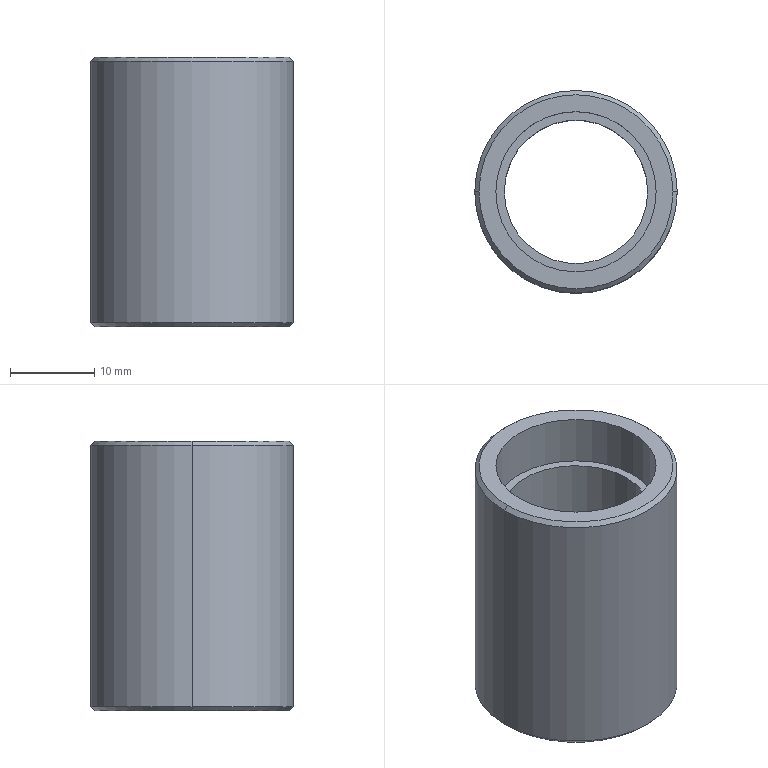Part | STEP file | QA-FC01 | 1 solid | 16 faces | box 24 x 24 x 32 mm | volume 6516 mm3 | cylinder 8 | cone 4 | plane 4 | commonest cylinder face diameters 19 x4 17 x2 24 x2
STEP:
#1=CARTESIAN_POINT('',(0.,0.,0.));
#2=DIRECTION('',(0.,0.,1.));
#3=DIRECTION('',(1.,0.,0.));
#4=AXIS2_PLACEMENT_3D('',#1,#2,#3);
#5=CARTESIAN_POINT('',(11.5,0.,32.));
#6=VERTEX_POINT('',#5);
#7=CARTESIAN_POINT('',(-11.5,0.,32.));
#8=VERTEX_POINT('',#7);
#9=CARTESIAN_POINT('',(0.,0.,32.));
#10=DIRECTION('',(0.,0.,1.));
#11=DIRECTION('',(1.,0.,0.));
#12=AXIS2_PLACEMENT_3D('',#9,#10,#11);
#13=CIRCLE('',#12,11.5);
#14=CARTESIAN_POINT('',(0.,0.,32.));
#15=DIRECTION('',(0.,0.,-1.));
#16=DIRECTION('',(-1.,0.,0.));
#17=AXIS2_PLACEMENT_3D('',#14,#15,#16);
#18=CONICAL_SURFACE('',#17,11.5,0.7854);
#19=CARTESIAN_POINT('',(3.142,0.));
#20=DIRECTION('',(-1.,0.));
#21=VECTOR('',#20,1.);
#22=LINE('',#19,#21);
#23=(GEOMETRIC_REPRESENTATION_CONTEXT(2)PARAMETRIC_REPRESENTATION_CONTEXT()REPRESENTATION_CONTEXT('',''));
#24=DEFINITIONAL_REPRESENTATION('',(#22),#23);
#25=PCURVE('',#18,#24);
#26=CARTESIAN_POINT('',(0.,0.,32.));
#27=DIRECTION('',(0.,0.,1.));
#28=DIRECTION('',(1.,0.,0.));
#29=AXIS2_PLACEMENT_3D('',#26,#27,#28);
#30=PLANE('',#29);
#31=CARTESIAN_POINT('',(0.,0.));
#32=DIRECTION('',(1.,0.));
#33=AXIS2_PLACEMENT_2D('',#31,#32);
#34=CIRCLE('',#33,11.5);
#35=(GEOMETRIC_REPRESENTATION_CONTEXT(2)PARAMETRIC_REPRESENTATION_CONTEXT()REPRESENTATION_CONTEXT('',''));
#36=DEFINITIONAL_REPRESENTATION('',(#34),#35);
#37=PCURVE('',#30,#36);
#38=SURFACE_CURVE('',#13,(#25,#37),.PCURVE_S1.);
#39=EDGE_CURVE('',#6,#8,#38,.T.);
#40=ORIENTED_EDGE('',*,*,#39,.F.);
#41=CARTESIAN_POINT('',(12.,0.,31.5));
#42=VERTEX_POINT('',#41);
#43=CARTESIAN_POINT('',(11.5,0.,32.));
#44=DIRECTION('',(0.7071,0.,-0.7071));
#45=VECTOR('',#44,1.);
#46=LINE('',#43,#45);
#47=CARTESIAN_POINT('',(3.142,0.));
#48=DIRECTION('',(0.,1.));
#49=VECTOR('',#48,1.);
#50=LINE('',#47,#49);
#51=(GEOMETRIC_REPRESENTATION_CONTEXT(2)PARAMETRIC_REPRESENTATION_CONTEXT()REPRESENTATION_CONTEXT('',''));
#52=DEFINITIONAL_REPRESENTATION('',(#50),#51);
#53=PCURVE('',#18,#52);
#54=CARTESIAN_POINT('',(0.,0.,32.));
#55=DIRECTION('',(0.,0.,-1.));
#56=DIRECTION('',(-1.,0.,0.));
#57=AXIS2_PLACEMENT_3D('',#54,#55,#56);
#58=CONICAL_SURFACE('',#57,11.5,0.7854);
#59=CARTESIAN_POINT('',(3.142,0.));
#60=DIRECTION('',(0.,1.));
#61=VECTOR('',#60,1.);
#62=LINE('',#59,#61);
#63=(GEOMETRIC_REPRESENTATION_CONTEXT(2)PARAMETRIC_REPRESENTATION_CONTEXT()REPRESENTATION_CONTEXT('',''));
#64=DEFINITIONAL_REPRESENTATION('',(#62),#63);
#65=PCURVE('',#58,#64);
#66=SURFACE_CURVE('',#46,(#53,#65),.PCURVE_S1.);
#67=EDGE_CURVE('',#6,#42,#66,.T.);
#68=ORIENTED_EDGE('',*,*,#67,.T.);
#69=CARTESIAN_POINT('',(-12.,0.,31.5));
#70=VERTEX_POINT('',#69);
#71=CARTESIAN_POINT('',(0.,0.,31.5));
#72=DIRECTION('',(0.,0.,-1.));
#73=DIRECTION('',(1.,0.,0.));
#74=AXIS2_PLACEMENT_3D('',#71,#72,#73);
#75=CIRCLE('',#74,12.);
#76=CARTESIAN_POINT('',(-3.142,0.5));
#77=DIRECTION('',(1.,0.));
#78=VECTOR('',#77,1.);
#79=LINE('',#76,#78);
#80=(GEOMETRIC_REPRESENTATION_CONTEXT(2)PARAMETRIC_REPRESENTATION_CONTEXT()REPRESENTATION_CONTEXT('',''));
#81=DEFINITIONAL_REPRESENTATION('',(#79),#80);
#82=PCURVE('',#18,#81);
#83=CARTESIAN_POINT('',(0.,0.,32.));
#84=DIRECTION('',(0.,0.,-1.));
#85=DIRECTION('',(-1.,0.,0.));
#86=AXIS2_PLACEMENT_3D('',#83,#84,#85);
#87=CYLINDRICAL_SURFACE('',#86,12.);
#88=CARTESIAN_POINT('',(-3.142,0.5));
#89=DIRECTION('',(1.,0.));
#90=VECTOR('',#89,1.);
#91=LINE('',#88,#90);
#92=(GEOMETRIC_REPRESENTATION_CONTEXT(2)PARAMETRIC_REPRESENTATION_CONTEXT()REPRESENTATION_CONTEXT('',''));
#93=DEFINITIONAL_REPRESENTATION('',(#91),#92);
#94=PCURVE('',#87,#93);
#95=SURFACE_CURVE('',#75,(#82,#94),.PCURVE_S1.);
#96=EDGE_CURVE('',#70,#42,#95,.T.);
#97=ORIENTED_EDGE('',*,*,#96,.F.);
#98=CARTESIAN_POINT('',(-11.5,0.,32.));
#99=DIRECTION('',(-0.7071,0.,-0.7071));
#100=VECTOR('',#99,1.);
#101=LINE('',#98,#100);
#102=CARTESIAN_POINT('',(0.,0.));
#103=DIRECTION('',(0.,1.));
#104=VECTOR('',#103,1.);
#105=LINE('',#102,#104);
#106=(GEOMETRIC_REPRESENTATION_CONTEXT(2)PARAMETRIC_REPRESENTATION_CONTEXT()REPRESENTATION_CONTEXT('',''));
#107=DEFINITIONAL_REPRESENTATION('',(#105),#106);
#108=PCURVE('',#18,#107);
#109=CARTESIAN_POINT('',(6.283,0.));
#110=DIRECTION('',(0.,1.));
#111=VECTOR('',#110,1.);
#112=LINE('',#109,#111);
#113=(GEOMETRIC_REPRESENTATION_CONTEXT(2)PARAMETRIC_REPRESENTATION_CONTEXT()REPRESENTATION_CONTEXT('',''));
#114=DEFINITIONAL_REPRESENTATION('',(#112),#113);
#115=PCURVE('',#58,#114);
#116=SURFACE_CURVE('',#101,(#108,#115),.PCURVE_S1.);
#117=EDGE_CURVE('',#8,#70,#116,.T.);
#118=ORIENTED_EDGE('',*,*,#117,.F.);
#119=EDGE_LOOP('',(#40,#68,#97,#118));
#120=FACE_BOUND('',#119,.T.);
#121=ADVANCED_FACE('',(#120),#18,.T.);
#122=CARTESIAN_POINT('',(-11.5,0.,0.));
#123=VERTEX_POINT('',#122);
#124=CARTESIAN_POINT('',(11.5,0.,0.));
#125=VERTEX_POINT('',#124);
#126=CARTESIAN_POINT('',(0.,0.,0.));
#127=DIRECTION('',(0.,0.,-1.));
#128=DIRECTION('',(1.,0.,0.));
#129=AXIS2_PLACEMENT_3D('',#126,#127,#128);
#130=CIRCLE('',#129,11.5);
#131=CARTESIAN_POINT('',(0.,0.,0.5));
#132=DIRECTION('',(0.,0.,1.));
#133=DIRECTION('',(1.,0.,0.));
#134=AXIS2_PLACEMENT_3D('',#131,#132,#133);
#135=CONICAL_SURFACE('',#134,12.,0.7854);
#136=CARTESIAN_POINT('',(6.283,-0.5));
#137=DIRECTION('',(-1.,0.));
#138=VECTOR('',#137,1.);
#139=LINE('',#136,#138);
#140=(GEOMETRIC_REPRESENTATION_CONTEXT(2)PARAMETRIC_REPRESENTATION_CONTEXT()REPRESENTATION_CONTEXT('',''));
#141=DEFINITIONAL_REPRESENTATION('',(#139),#140);
#142=PCURVE('',#135,#141);
#143=CARTESIAN_POINT('',(0.,0.,0.));
#144=DIRECTION('',(0.,0.,1.));
#145=DIRECTION('',(1.,0.,0.));
#146=AXIS2_PLACEMENT_3D('',#143,#144,#145);
#147=PLANE('',#146);
#148=CARTESIAN_POINT('',(11.5,0.));
#149=CARTESIAN_POINT('',(11.5,-19.919));
#150=CARTESIAN_POINT('',(-5.75,-9.959));
#151=CARTESIAN_POINT('',(-23.,0.));
#152=CARTESIAN_POINT('',(-5.75,9.959));
#153=CARTESIAN_POINT('',(11.5,19.919));
#154=CARTESIAN_POINT('',(11.5,0.));
#155=(BOUNDED_CURVE()B_SPLINE_CURVE(2,(#148,#149,#150,#151,#152,#153,#154),.UNSPECIFIED.,.T.,.F.)B_SPLINE_CURVE_WITH_KNOTS((1,2,2,2,2,1),(-2.094,0.,2.094,4.189,6.283,8.378),.UNSPECIFIED.)CURVE()GEOMETRIC_REPRESENTATION_ITEM()RATIONAL_B_SPLINE_CURVE((1.,0.5,1.,0.5,1.,0.5,1.))REPRESENTATION_ITEM(''));
#156=(GEOMETRIC_REPRESENTATION_CONTEXT(2)PARAMETRIC_REPRESENTATION_CONTEXT()REPRESENTATION_CONTEXT('',''));
#157=DEFINITIONAL_REPRESENTATION('',(#155),#156);
#158=PCURVE('',#147,#157);
#159=SURFACE_CURVE('',#130,(#142,#158),.PCURVE_S1.);
#160=EDGE_CURVE('',#123,#125,#159,.T.);
#161=ORIENTED_EDGE('',*,*,#160,.F.);
#162=CARTESIAN_POINT('',(-12.,0.,0.5));
#163=VERTEX_POINT('',#162);
#164=CARTESIAN_POINT('',(-12.,0.,0.5));
#165=DIRECTION('',(-0.7071,0.,0.7071));
#166=VECTOR('',#165,1.);
#167=LINE('',#164,#166);
#168=CARTESIAN_POINT('',(3.142,0.));
#169=DIRECTION('',(0.,1.));
#170=VECTOR('',#169,1.);
#171=LINE('',#168,#170);
#172=(GEOMETRIC_REPRESENTATION_CONTEXT(2)PARAMETRIC_REPRESENTATION_CONTEXT()REPRESENTATION_CONTEXT('',''));
#173=DEFINITIONAL_REPRESENTATION('',(#171),#172);
#174=PCURVE('',#135,#173);
#175=CARTESIAN_POINT('',(0.,0.,0.5));
#176=DIRECTION('',(0.,0.,1.));
#177=DIRECTION('',(1.,0.,0.));
#178=AXIS2_PLACEMENT_3D('',#175,#176,#177);
#179=CONICAL_SURFACE('',#178,12.,0.7854);
#180=CARTESIAN_POINT('',(3.142,0.));
#181=DIRECTION('',(0.,1.));
#182=VECTOR('',#181,1.);
#183=LINE('',#180,#182);
#184=(GEOMETRIC_REPRESENTATION_CONTEXT(2)PARAMETRIC_REPRESENTATION_CONTEXT()REPRESENTATION_CONTEXT('',''));
#185=DEFINITIONAL_REPRESENTATION('',(#183),#184);
#186=PCURVE('',#179,#185);
#187=SURFACE_CURVE('',#167,(#174,#186),.PCURVE_S1.);
#188=EDGE_CURVE('',#123,#163,#187,.T.);
#189=ORIENTED_EDGE('',*,*,#188,.T.);
#190=CARTESIAN_POINT('',(12.,0.,0.5));
#191=VERTEX_POINT('',#190);
#192=CARTESIAN_POINT('',(0.,0.,0.5));
#193=DIRECTION('',(0.,0.,1.));
#194=DIRECTION('',(1.,0.,0.));
#195=AXIS2_PLACEMENT_3D('',#192,#193,#194);
#196=CIRCLE('',#195,12.);
#197=CARTESIAN_POINT('',(0.,0.));
#198=DIRECTION('',(1.,0.));
#199=VECTOR('',#198,1.);
#200=LINE('',#197,#199);
#201=(GEOMETRIC_REPRESENTATION_CONTEXT(2)PARAMETRIC_REPRESENTATION_CONTEXT()REPRESENTATION_CONTEXT('',''));
#202=DEFINITIONAL_REPRESENTATION('',(#200),#201);
#203=PCURVE('',#135,#202);
#204=CARTESIAN_POINT('',(3.142,31.5));
#205=DIRECTION('',(-1.,0.));
#206=VECTOR('',#205,1.);
#207=LINE('',#204,#206);
#208=(GEOMETRIC_REPRESENTATION_CONTEXT(2)PARAMETRIC_REPRESENTATION_CONTEXT()REPRESENTATION_CONTEXT('',''));
#209=DEFINITIONAL_REPRESENTATION('',(#207),#208);
#210=PCURVE('',#87,#209);
#211=SURFACE_CURVE('',#196,(#203,#210),.PCURVE_S1.);
#212=EDGE_CURVE('',#191,#163,#211,.T.);
#213=ORIENTED_EDGE('',*,*,#212,.F.);
#214=CARTESIAN_POINT('',(12.,0.,0.5));
#215=DIRECTION('',(0.7071,0.,0.7071));
#216=VECTOR('',#215,1.);
#217=LINE('',#214,#216);
#218=CARTESIAN_POINT('',(0.,0.));
#219=DIRECTION('',(0.,1.));
#220=VECTOR('',#219,1.);
#221=LINE('',#218,#220);
#222=(GEOMETRIC_REPRESENTATION_CONTEXT(2)PARAMETRIC_REPRESENTATION_CONTEXT()REPRESENTATION_CONTEXT('',''));
#223=DEFINITIONAL_REPRESENTATION('',(#221),#222);
#224=PCURVE('',#135,#223);
#225=CARTESIAN_POINT('',(6.283,0.));
#226=DIRECTION('',(0.,1.));
#227=VECTOR('',#226,1.);
#228=LINE('',#225,#227);
#229=(GEOMETRIC_REPRESENTATION_CONTEXT(2)PARAMETRIC_REPRESENTATION_CONTEXT()REPRESENTATION_CONTEXT('',''));
#230=DEFINITIONAL_REPRESENTATION('',(#228),#229);
#231=PCURVE('',#179,#230);
#232=SURFACE_CURVE('',#217,(#224,#231),.PCURVE_S1.);
#233=EDGE_CURVE('',#125,#191,#232,.T.);
#234=ORIENTED_EDGE('',*,*,#233,.F.);
#235=EDGE_LOOP('',(#161,#189,#213,#234));
#236=FACE_BOUND('',#235,.T.);
#237=ADVANCED_FACE('',(#236),#135,.T.);
#238=CARTESIAN_POINT('',(-9.5,0.,6.));
#239=VERTEX_POINT('',#238);
#240=CARTESIAN_POINT('',(-9.5,0.,0.));
#241=VERTEX_POINT('',#240);
#242=CARTESIAN_POINT('',(-9.5,0.,6.));
#243=DIRECTION('',(0.,0.,-1.));
#244=VECTOR('',#243,1.);
#245=LINE('',#242,#244);
#246=CARTESIAN_POINT('',(0.,0.,6.));
#247=DIRECTION('',(0.,0.,-1.));
#248=DIRECTION('',(-1.,0.,0.));
#249=AXIS2_PLACEMENT_3D('',#246,#247,#248);
#250=CYLINDRICAL_SURFACE('',#249,9.5);
#251=CARTESIAN_POINT('',(6.283,0.));
#252=DIRECTION('',(0.,1.));
#253=VECTOR('',#252,1.);
#254=LINE('',#251,#253);
#255=(GEOMETRIC_REPRESENTATION_CONTEXT(2)PARAMETRIC_REPRESENTATION_CONTEXT()REPRESENTATION_CONTEXT('',''));
#256=DEFINITIONAL_REPRESENTATION('',(#254),#255);
#257=PCURVE('',#250,#256);
#258=CARTESIAN_POINT('',(0.,0.,6.));
#259=DIRECTION('',(0.,0.,-1.));
#260=DIRECTION('',(-1.,0.,0.));
#261=AXIS2_PLACEMENT_3D('',#258,#259,#260);
#262=CYLINDRICAL_SURFACE('',#261,9.5);
#263=CARTESIAN_POINT('',(0.,0.));
#264=DIRECTION('',(0.,1.));
#265=VECTOR('',#264,1.);
#266=LINE('',#263,#265);
#267=(GEOMETRIC_REPRESENTATION_CONTEXT(2)PARAMETRIC_REPRESENTATION_CONTEXT()REPRESENTATION_CONTEXT('',''));
#268=DEFINITIONAL_REPRESENTATION('',(#266),#267);
#269=PCURVE('',#262,#268);
#270=SURFACE_CURVE('',#245,(#257,#269),.PCURVE_S1.);
#271=EDGE_CURVE('',#239,#241,#270,.T.);
#272=ORIENTED_EDGE('',*,*,#271,.T.);
#273=CARTESIAN_POINT('',(9.5,0.,0.));
#274=VERTEX_POINT('',#273);
#275=CARTESIAN_POINT('',(0.,0.,0.));
#276=DIRECTION('',(0.,0.,-1.));
#277=DIRECTION('',(-1.,0.,0.));
#278=AXIS2_PLACEMENT_3D('',#275,#276,#277);
#279=CIRCLE('',#278,9.5);
#280=CARTESIAN_POINT('',(0.,6.));
#281=DIRECTION('',(1.,0.));
#282=VECTOR('',#281,1.);
#283=LINE('',#280,#282);
#284=(GEOMETRIC_REPRESENTATION_CONTEXT(2)PARAMETRIC_REPRESENTATION_CONTEXT()REPRESENTATION_CONTEXT('',''));
#285=DEFINITIONAL_REPRESENTATION('',(#283),#284);
#286=PCURVE('',#250,#285);
#287=CARTESIAN_POINT('',(-9.5,0.));
#288=CARTESIAN_POINT('',(-9.5,16.454));
#289=CARTESIAN_POINT('',(4.75,8.227));
#290=CARTESIAN_POINT('',(19.,0.));
#291=CARTESIAN_POINT('',(4.75,-8.227));
#292=CARTESIAN_POINT('',(-9.5,-16.454));
#293=CARTESIAN_POINT('',(-9.5,0.));
#294=(BOUNDED_CURVE()B_SPLINE_CURVE(2,(#287,#288,#289,#290,#291,#292,#293),.UNSPECIFIED.,.T.,.F.)B_SPLINE_CURVE_WITH_KNOTS((1,2,2,2,2,1),(-2.094,0.,2.094,4.189,6.283,8.378),.UNSPECIFIED.)CURVE()GEOMETRIC_REPRESENTATION_ITEM()RATIONAL_B_SPLINE_CURVE((1.,0.5,1.,0.5,1.,0.5,1.))REPRESENTATION_ITEM(''));
#295=(GEOMETRIC_REPRESENTATION_CONTEXT(2)PARAMETRIC_REPRESENTATION_CONTEXT()REPRESENTATION_CONTEXT('',''));
#296=DEFINITIONAL_REPRESENTATION('',(#294),#295);
#297=PCURVE('',#147,#296);
#298=SURFACE_CURVE('',#279,(#286,#297),.PCURVE_S1.);
#299=EDGE_CURVE('',#274,#241,#298,.T.);
#300=ORIENTED_EDGE('',*,*,#299,.F.);
#301=CARTESIAN_POINT('',(9.5,0.,6.));
#302=VERTEX_POINT('',#301);
#303=CARTESIAN_POINT('',(9.5,0.,6.));
#304=DIRECTION('',(0.,0.,-1.));
#305=VECTOR('',#304,1.);
#306=LINE('',#303,#305);
#307=CARTESIAN_POINT('',(3.142,0.));
#308=DIRECTION('',(0.,1.));
#309=VECTOR('',#308,1.);
#310=LINE('',#307,#309);
#311=(GEOMETRIC_REPRESENTATION_CONTEXT(2)PARAMETRIC_REPRESENTATION_CONTEXT()REPRESENTATION_CONTEXT('',''));
#312=DEFINITIONAL_REPRESENTATION('',(#310),#311);
#313=PCURVE('',#250,#312);
#314=CARTESIAN_POINT('',(3.142,0.));
#315=DIRECTION('',(0.,1.));
#316=VECTOR('',#315,1.);
#317=LINE('',#314,#316);
#318=(GEOMETRIC_REPRESENTATION_CONTEXT(2)PARAMETRIC_REPRESENTATION_CONTEXT()REPRESENTATION_CONTEXT('',''));
#319=DEFINITIONAL_REPRESENTATION('',(#317),#318);
#320=PCURVE('',#262,#319);
#321=SURFACE_CURVE('',#306,(#313,#320),.PCURVE_S1.);
#322=EDGE_CURVE('',#302,#274,#321,.T.);
#323=ORIENTED_EDGE('',*,*,#322,.F.);
#324=CARTESIAN_POINT('',(0.,0.,6.));
#325=DIRECTION('',(0.,0.,-1.));
#326=DIRECTION('',(-1.,0.,0.));
#327=AXIS2_PLACEMENT_3D('',#324,#325,#326);
#328=CIRCLE('',#327,9.5);
#329=CARTESIAN_POINT('',(0.,0.));
#330=DIRECTION('',(1.,0.));
#331=VECTOR('',#330,1.);
#332=LINE('',#329,#331);
#333=(GEOMETRIC_REPRESENTATION_CONTEXT(2)PARAMETRIC_REPRESENTATION_CONTEXT()REPRESENTATION_CONTEXT('',''));
#334=DEFINITIONAL_REPRESENTATION('',(#332),#333);
#335=PCURVE('',#250,#334);
#336=CARTESIAN_POINT('',(0.,0.,6.));
#337=DIRECTION('',(0.,0.,-1.));
#338=DIRECTION('',(-1.,0.,0.));
#339=AXIS2_PLACEMENT_3D('',#336,#337,#338);
#340=PLANE('',#339);
#341=CARTESIAN_POINT('',(0.,0.));
#342=DIRECTION('',(1.,0.));
#343=AXIS2_PLACEMENT_2D('',#341,#342);
#344=CIRCLE('',#343,9.5);
#345=(GEOMETRIC_REPRESENTATION_CONTEXT(2)PARAMETRIC_REPRESENTATION_CONTEXT()REPRESENTATION_CONTEXT('',''));
#346=DEFINITIONAL_REPRESENTATION('',(#344),#345);
#347=PCURVE('',#340,#346);
#348=SURFACE_CURVE('',#328,(#335,#347),.PCURVE_S1.);
#349=EDGE_CURVE('',#302,#239,#348,.T.);
#350=ORIENTED_EDGE('',*,*,#349,.T.);
#351=EDGE_LOOP('',(#272,#300,#323,#350));
#352=FACE_BOUND('',#351,.F.);
#353=ADVANCED_FACE('',(#352),#250,.F.);
#354=CARTESIAN_POINT('',(9.5,0.,26.));
#355=VERTEX_POINT('',#354);
#356=CARTESIAN_POINT('',(9.5,0.,32.));
#357=VERTEX_POINT('',#356);
#358=CARTESIAN_POINT('',(9.5,0.,26.));
#359=DIRECTION('',(0.,0.,1.));
#360=VECTOR('',#359,1.);
#361=LINE('',#358,#360);
#362=CARTESIAN_POINT('',(0.,0.,26.));
#363=DIRECTION('',(0.,0.,1.));
#364=DIRECTION('',(1.,0.,0.));
#365=AXIS2_PLACEMENT_3D('',#362,#363,#364);
#366=CYLINDRICAL_SURFACE('',#365,9.5);
#367=CARTESIAN_POINT('',(6.283,0.));
#368=DIRECTION('',(0.,1.));
#369=VECTOR('',#368,1.);
#370=LINE('',#367,#369);
#371=(GEOMETRIC_REPRESENTATION_CONTEXT(2)PARAMETRIC_REPRESENTATION_CONTEXT()REPRESENTATION_CONTEXT('',''));
#372=DEFINITIONAL_REPRESENTATION('',(#370),#371);
#373=PCURVE('',#366,#372);
#374=CARTESIAN_POINT('',(0.,0.,26.));
#375=DIRECTION('',(0.,0.,1.));
#376=DIRECTION('',(1.,0.,0.));
#377=AXIS2_PLACEMENT_3D('',#374,#375,#376);
#378=CYLINDRICAL_SURFACE('',#377,9.5);
#379=CARTESIAN_POINT('',(0.,0.));
#380=DIRECTION('',(0.,1.));
#381=VECTOR('',#380,1.);
#382=LINE('',#379,#381);
#383=(GEOMETRIC_REPRESENTATION_CONTEXT(2)PARAMETRIC_REPRESENTATION_CONTEXT()REPRESENTATION_CONTEXT('',''));
#384=DEFINITIONAL_REPRESENTATION('',(#382),#383);
#385=PCURVE('',#378,#384);
#386=SURFACE_CURVE('',#361,(#373,#385),.PCURVE_S1.);
#387=EDGE_CURVE('',#355,#357,#386,.T.);
#388=ORIENTED_EDGE('',*,*,#387,.T.);
#389=CARTESIAN_POINT('',(-9.5,0.,32.));
#390=VERTEX_POINT('',#389);
#391=CARTESIAN_POINT('',(0.,0.,32.));
#392=DIRECTION('',(0.,0.,1.));
#393=DIRECTION('',(1.,0.,0.));
#394=AXIS2_PLACEMENT_3D('',#391,#392,#393);
#395=CIRCLE('',#394,9.5);
#396=CARTESIAN_POINT('',(0.,6.));
#397=DIRECTION('',(1.,0.));
#398=VECTOR('',#397,1.);
#399=LINE('',#396,#398);
#400=(GEOMETRIC_REPRESENTATION_CONTEXT(2)PARAMETRIC_REPRESENTATION_CONTEXT()REPRESENTATION_CONTEXT('',''));
#401=DEFINITIONAL_REPRESENTATION('',(#399),#400);
#402=PCURVE('',#366,#401);
#403=CARTESIAN_POINT('',(0.,0.));
#404=DIRECTION('',(1.,0.));
#405=AXIS2_PLACEMENT_2D('',#403,#404);
#406=CIRCLE('',#405,9.5);
#407=(GEOMETRIC_REPRESENTATION_CONTEXT(2)PARAMETRIC_REPRESENTATION_CONTEXT()REPRESENTATION_CONTEXT('',''));
#408=DEFINITIONAL_REPRESENTATION('',(#406),#407);
#409=PCURVE('',#30,#408);
#410=SURFACE_CURVE('',#395,(#402,#409),.PCURVE_S1.);
#411=EDGE_CURVE('',#390,#357,#410,.T.);
#412=ORIENTED_EDGE('',*,*,#411,.F.);
#413=CARTESIAN_POINT('',(-9.5,0.,26.));
#414=VERTEX_POINT('',#413);
#415=CARTESIAN_POINT('',(-9.5,0.,26.));
#416=DIRECTION('',(0.,0.,1.));
#417=VECTOR('',#416,1.);
#418=LINE('',#415,#417);
#419=CARTESIAN_POINT('',(3.142,0.));
#420=DIRECTION('',(0.,1.));
#421=VECTOR('',#420,1.);
#422=LINE('',#419,#421);
#423=(GEOMETRIC_REPRESENTATION_CONTEXT(2)PARAMETRIC_REPRESENTATION_CONTEXT()REPRESENTATION_CONTEXT('',''));
#424=DEFINITIONAL_REPRESENTATION('',(#422),#423);
#425=PCURVE('',#366,#424);
#426=CARTESIAN_POINT('',(3.142,0.));
#427=DIRECTION('',(0.,1.));
#428=VECTOR('',#427,1.);
#429=LINE('',#426,#428);
#430=(GEOMETRIC_REPRESENTATION_CONTEXT(2)PARAMETRIC_REPRESENTATION_CONTEXT()REPRESENTATION_CONTEXT('',''));
#431=DEFINITIONAL_REPRESENTATION('',(#429),#430);
#432=PCURVE('',#378,#431);
#433=SURFACE_CURVE('',#418,(#425,#432),.PCURVE_S1.);
#434=EDGE_CURVE('',#414,#390,#433,.T.);
#435=ORIENTED_EDGE('',*,*,#434,.F.);
#436=CARTESIAN_POINT('',(0.,0.,26.));
#437=DIRECTION('',(0.,0.,1.));
#438=DIRECTION('',(1.,0.,0.));
#439=AXIS2_PLACEMENT_3D('',#436,#437,#438);
#440=CIRCLE('',#439,9.5);
#441=CARTESIAN_POINT('',(0.,0.));
#442=DIRECTION('',(1.,0.));
#443=VECTOR('',#442,1.);
#444=LINE('',#441,#443);
#445=(GEOMETRIC_REPRESENTATION_CONTEXT(2)PARAMETRIC_REPRESENTATION_CONTEXT()REPRESENTATION_CONTEXT('',''));
#446=DEFINITIONAL_REPRESENTATION('',(#444),#445);
#447=PCURVE('',#366,#446);
#448=CARTESIAN_POINT('',(0.,0.,26.));
#449=DIRECTION('',(0.,0.,1.));
#450=DIRECTION('',(1.,0.,0.));
#451=AXIS2_PLACEMENT_3D('',#448,#449,#450);
#452=PLANE('',#451);
#453=CARTESIAN_POINT('',(0.,0.));
#454=DIRECTION('',(1.,0.));
#455=AXIS2_PLACEMENT_2D('',#453,#454);
#456=CIRCLE('',#455,9.5);
#457=(GEOMETRIC_REPRESENTATION_CONTEXT(2)PARAMETRIC_REPRESENTATION_CONTEXT()REPRESENTATION_CONTEXT('',''));
#458=DEFINITIONAL_REPRESENTATION('',(#456),#457);
#459=PCURVE('',#452,#458);
#460=SURFACE_CURVE('',#440,(#447,#459),.PCURVE_S1.);
#461=EDGE_CURVE('',#414,#355,#460,.T.);
#462=ORIENTED_EDGE('',*,*,#461,.T.);
#463=EDGE_LOOP('',(#388,#412,#435,#462));
#464=FACE_BOUND('',#463,.F.);
#465=ADVANCED_FACE('',(#464),#366,.F.);
#466=ORIENTED_EDGE('',*,*,#96,.T.);
#467=CARTESIAN_POINT('',(12.,0.,32.));
#468=DIRECTION('',(0.,0.,-1.));
#469=VECTOR('',#468,1.);
#470=LINE('',#467,#469);
#471=CARTESIAN_POINT('',(3.142,0.));
#472=DIRECTION('',(0.,1.));
#473=VECTOR('',#472,1.);
#474=LINE('',#471,#473);
#475=(GEOMETRIC_REPRESENTATION_CONTEXT(2)PARAMETRIC_REPRESENTATION_CONTEXT()REPRESENTATION_CONTEXT('',''));
#476=DEFINITIONAL_REPRESENTATION('',(#474),#475);
#477=PCURVE('',#87,#476);
#478=CARTESIAN_POINT('',(0.,0.,32.));
#479=DIRECTION('',(0.,0.,-1.));
#480=DIRECTION('',(-1.,0.,0.));
#481=AXIS2_PLACEMENT_3D('',#478,#479,#480);
#482=CYLINDRICAL_SURFACE('',#481,12.);
#483=CARTESIAN_POINT('',(3.142,0.));
#484=DIRECTION('',(0.,1.));
#485=VECTOR('',#484,1.);
#486=LINE('',#483,#485);
#487=(GEOMETRIC_REPRESENTATION_CONTEXT(2)PARAMETRIC_REPRESENTATION_CONTEXT()REPRESENTATION_CONTEXT('',''));
#488=DEFINITIONAL_REPRESENTATION('',(#486),#487);
#489=PCURVE('',#482,#488);
#490=SURFACE_CURVE('',#470,(#477,#489),.PCURVE_S1.);
#491=EDGE_CURVE('',#42,#191,#490,.T.);
#492=ORIENTED_EDGE('',*,*,#491,.T.);
#493=ORIENTED_EDGE('',*,*,#212,.T.);
#494=CARTESIAN_POINT('',(-12.,0.,32.));
#495=DIRECTION('',(0.,0.,-1.));
#496=VECTOR('',#495,1.);
#497=LINE('',#494,#496);
#498=CARTESIAN_POINT('',(0.,0.));
#499=DIRECTION('',(0.,1.));
#500=VECTOR('',#499,1.);
#501=LINE('',#498,#500);
#502=(GEOMETRIC_REPRESENTATION_CONTEXT(2)PARAMETRIC_REPRESENTATION_CONTEXT()REPRESENTATION_CONTEXT('',''));
#503=DEFINITIONAL_REPRESENTATION('',(#501),#502);
#504=PCURVE('',#87,#503);
#505=CARTESIAN_POINT('',(6.283,0.));
#506=DIRECTION('',(0.,1.));
#507=VECTOR('',#506,1.);
#508=LINE('',#505,#507);
#509=(GEOMETRIC_REPRESENTATION_CONTEXT(2)PARAMETRIC_REPRESENTATION_CONTEXT()REPRESENTATION_CONTEXT('',''));
#510=DEFINITIONAL_REPRESENTATION('',(#508),#509);
#511=PCURVE('',#482,#510);
#512=SURFACE_CURVE('',#497,(#504,#511),.PCURVE_S1.);
#513=EDGE_CURVE('',#70,#163,#512,.T.);
#514=ORIENTED_EDGE('',*,*,#513,.F.);
#515=EDGE_LOOP('',(#466,#492,#493,#514));
#516=FACE_BOUND('',#515,.T.);
#517=ADVANCED_FACE('',(#516),#87,.T.);
#518=CARTESIAN_POINT('',(8.5,0.,6.));
#519=VERTEX_POINT('',#518);
#520=CARTESIAN_POINT('',(8.5,0.,26.));
#521=VERTEX_POINT('',#520);
#522=CARTESIAN_POINT('',(8.5,0.,0.));
#523=DIRECTION('',(0.,0.,1.));
#524=VECTOR('',#523,1.);
#525=LINE('',#522,#524);
#526=CARTESIAN_POINT('',(0.,0.,0.));
#527=DIRECTION('',(0.,0.,1.));
#528=DIRECTION('',(1.,0.,0.));
#529=AXIS2_PLACEMENT_3D('',#526,#527,#528);
#530=CYLINDRICAL_SURFACE('',#529,8.5);
#531=CARTESIAN_POINT('',(6.283,0.));
#532=DIRECTION('',(0.,1.));
#533=VECTOR('',#532,1.);
#534=LINE('',#531,#533);
#535=(GEOMETRIC_REPRESENTATION_CONTEXT(2)PARAMETRIC_REPRESENTATION_CONTEXT()REPRESENTATION_CONTEXT('',''));
#536=DEFINITIONAL_REPRESENTATION('',(#534),#535);
#537=PCURVE('',#530,#536);
#538=CARTESIAN_POINT('',(0.,0.,0.));
#539=DIRECTION('',(0.,0.,1.));
#540=DIRECTION('',(1.,0.,0.));
#541=AXIS2_PLACEMENT_3D('',#538,#539,#540);
#542=CYLINDRICAL_SURFACE('',#541,8.5);
#543=CARTESIAN_POINT('',(0.,0.));
#544=DIRECTION('',(0.,1.));
#545=VECTOR('',#544,1.);
#546=LINE('',#543,#545);
#547=(GEOMETRIC_REPRESENTATION_CONTEXT(2)PARAMETRIC_REPRESENTATION_CONTEXT()REPRESENTATION_CONTEXT('',''));
#548=DEFINITIONAL_REPRESENTATION('',(#546),#547);
#549=PCURVE('',#542,#548);
#550=SURFACE_CURVE('',#525,(#537,#549),.PCURVE_S1.);
#551=EDGE_CURVE('',#519,#521,#550,.T.);
#552=ORIENTED_EDGE('',*,*,#551,.T.);
#553=CARTESIAN_POINT('',(-8.5,0.,26.));
#554=VERTEX_POINT('',#553);
#555=CARTESIAN_POINT('',(0.,0.,26.));
#556=DIRECTION('',(0.,0.,-1.));
#557=DIRECTION('',(1.,0.,0.));
#558=AXIS2_PLACEMENT_3D('',#555,#556,#557);
#559=CIRCLE('',#558,8.5);
#560=CARTESIAN_POINT('',(6.283,26.));
#561=DIRECTION('',(-1.,0.));
#562=VECTOR('',#561,1.);
#563=LINE('',#560,#562);
#564=(GEOMETRIC_REPRESENTATION_CONTEXT(2)PARAMETRIC_REPRESENTATION_CONTEXT()REPRESENTATION_CONTEXT('',''));
#565=DEFINITIONAL_REPRESENTATION('',(#563),#564);
#566=PCURVE('',#530,#565);
#567=CARTESIAN_POINT('',(8.5,0.));
#568=CARTESIAN_POINT('',(8.5,-14.722));
#569=CARTESIAN_POINT('',(-4.25,-7.361));
#570=CARTESIAN_POINT('',(-17.,0.));
#571=CARTESIAN_POINT('',(-4.25,7.361));
#572=CARTESIAN_POINT('',(8.5,14.722));
#573=CARTESIAN_POINT('',(8.5,0.));
#574=(BOUNDED_CURVE()B_SPLINE_CURVE(2,(#567,#568,#569,#570,#571,#572,#573),.UNSPECIFIED.,.T.,.F.)B_SPLINE_CURVE_WITH_KNOTS((1,2,2,2,2,1),(-2.094,0.,2.094,4.189,6.283,8.378),.UNSPECIFIED.)CURVE()GEOMETRIC_REPRESENTATION_ITEM()RATIONAL_B_SPLINE_CURVE((1.,0.5,1.,0.5,1.,0.5,1.))REPRESENTATION_ITEM(''));
#575=(GEOMETRIC_REPRESENTATION_CONTEXT(2)PARAMETRIC_REPRESENTATION_CONTEXT()REPRESENTATION_CONTEXT('',''));
#576=DEFINITIONAL_REPRESENTATION('',(#574),#575);
#577=PCURVE('',#452,#576);
#578=SURFACE_CURVE('',#559,(#566,#577),.PCURVE_S1.);
#579=EDGE_CURVE('',#521,#554,#578,.T.);
#580=ORIENTED_EDGE('',*,*,#579,.T.);
#581=CARTESIAN_POINT('',(-8.5,0.,6.));
#582=VERTEX_POINT('',#581);
#583=CARTESIAN_POINT('',(-8.5,0.,0.));
#584=DIRECTION('',(0.,0.,1.));
#585=VECTOR('',#584,1.);
#586=LINE('',#583,#585);
#587=CARTESIAN_POINT('',(3.142,0.));
#588=DIRECTION('',(0.,1.));
#589=VECTOR('',#588,1.);
#590=LINE('',#587,#589);
#591=(GEOMETRIC_REPRESENTATION_CONTEXT(2)PARAMETRIC_REPRESENTATION_CONTEXT()REPRESENTATION_CONTEXT('',''));
#592=DEFINITIONAL_REPRESENTATION('',(#590),#591);
#593=PCURVE('',#530,#592);
#594=CARTESIAN_POINT('',(3.142,0.));
#595=DIRECTION('',(0.,1.));
#596=VECTOR('',#595,1.);
#597=LINE('',#594,#596);
#598=(GEOMETRIC_REPRESENTATION_CONTEXT(2)PARAMETRIC_REPRESENTATION_CONTEXT()REPRESENTATION_CONTEXT('',''));
#599=DEFINITIONAL_REPRESENTATION('',(#597),#598);
#600=PCURVE('',#542,#599);
#601=SURFACE_CURVE('',#586,(#593,#600),.PCURVE_S1.);
#602=EDGE_CURVE('',#582,#554,#601,.T.);
#603=ORIENTED_EDGE('',*,*,#602,.F.);
#604=CARTESIAN_POINT('',(0.,0.,6.));
#605=DIRECTION('',(0.,0.,1.));
#606=DIRECTION('',(-1.,0.,0.));
#607=AXIS2_PLACEMENT_3D('',#604,#605,#606);
#608=CIRCLE('',#607,8.5);
#609=CARTESIAN_POINT('',(3.142,6.));
#610=DIRECTION('',(1.,0.));
#611=VECTOR('',#610,1.);
#612=LINE('',#609,#611);
#613=(GEOMETRIC_REPRESENTATION_CONTEXT(2)PARAMETRIC_REPRESENTATION_CONTEXT()REPRESENTATION_CONTEXT('',''));
#614=DEFINITIONAL_REPRESENTATION('',(#612),#613);
#615=PCURVE('',#530,#614);
#616=CARTESIAN_POINT('',(8.5,0.));
#617=CARTESIAN_POINT('',(8.5,-14.722));
#618=CARTESIAN_POINT('',(-4.25,-7.361));
#619=CARTESIAN_POINT('',(-17.,0.));
#620=CARTESIAN_POINT('',(-4.25,7.361));
#621=CARTESIAN_POINT('',(8.5,14.722));
#622=CARTESIAN_POINT('',(8.5,0.));
#623=(BOUNDED_CURVE()B_SPLINE_CURVE(2,(#616,#617,#618,#619,#620,#621,#622),.UNSPECIFIED.,.T.,.F.)B_SPLINE_CURVE_WITH_KNOTS((1,2,2,2,2,1),(-2.094,0.,2.094,4.189,6.283,8.378),.UNSPECIFIED.)CURVE()GEOMETRIC_REPRESENTATION_ITEM()RATIONAL_B_SPLINE_CURVE((1.,0.5,1.,0.5,1.,0.5,1.))REPRESENTATION_ITEM(''));
#624=(GEOMETRIC_REPRESENTATION_CONTEXT(2)PARAMETRIC_REPRESENTATION_CONTEXT()REPRESENTATION_CONTEXT('',''));
#625=DEFINITIONAL_REPRESENTATION('',(#623),#624);
#626=PCURVE('',#340,#625);
#627=SURFACE_CURVE('',#608,(#615,#626),.PCURVE_S1.);
#628=EDGE_CURVE('',#582,#519,#627,.T.);
#629=ORIENTED_EDGE('',*,*,#628,.T.);
#630=EDGE_LOOP('',(#552,#580,#603,#629));
#631=FACE_BOUND('',#630,.F.);
#632=ADVANCED_FACE('',(#631),#530,.F.);
#633=CARTESIAN_POINT('',(0.,0.,26.));
#634=DIRECTION('',(0.,0.,-1.));
#635=DIRECTION('',(1.,0.,0.));
#636=AXIS2_PLACEMENT_3D('',#633,#634,#635);
#637=CIRCLE('',#636,8.5);
#638=CARTESIAN_POINT('',(6.283,26.));
#639=DIRECTION('',(-1.,0.));
#640=VECTOR('',#639,1.);
#641=LINE('',#638,#640);
#642=(GEOMETRIC_REPRESENTATION_CONTEXT(2)PARAMETRIC_REPRESENTATION_CONTEXT()REPRESENTATION_CONTEXT('',''));
#643=DEFINITIONAL_REPRESENTATION('',(#641),#642);
#644=PCURVE('',#542,#643);
#645=CARTESIAN_POINT('',(8.5,0.));
#646=CARTESIAN_POINT('',(8.5,-14.722));
#647=CARTESIAN_POINT('',(-4.25,-7.361));
#648=CARTESIAN_POINT('',(-17.,0.));
#649=CARTESIAN_POINT('',(-4.25,7.361));
#650=CARTESIAN_POINT('',(8.5,14.722));
#651=CARTESIAN_POINT('',(8.5,0.));
#652=(BOUNDED_CURVE()B_SPLINE_CURVE(2,(#645,#646,#647,#648,#649,#650,#651),.UNSPECIFIED.,.T.,.F.)B_SPLINE_CURVE_WITH_KNOTS((1,2,2,2,2,1),(-2.094,0.,2.094,4.189,6.283,8.378),.UNSPECIFIED.)CURVE()GEOMETRIC_REPRESENTATION_ITEM()RATIONAL_B_SPLINE_CURVE((1.,0.5,1.,0.5,1.,0.5,1.))REPRESENTATION_ITEM(''));
#653=(GEOMETRIC_REPRESENTATION_CONTEXT(2)PARAMETRIC_REPRESENTATION_CONTEXT()REPRESENTATION_CONTEXT('',''));
#654=DEFINITIONAL_REPRESENTATION('',(#652),#653);
#655=PCURVE('',#452,#654);
#656=SURFACE_CURVE('',#637,(#644,#655),.PCURVE_S1.);
#657=EDGE_CURVE('',#554,#521,#656,.T.);
#658=ORIENTED_EDGE('',*,*,#657,.T.);
#659=ORIENTED_EDGE('',*,*,#551,.F.);
#660=CARTESIAN_POINT('',(0.,0.,6.));
#661=DIRECTION('',(0.,0.,1.));
#662=DIRECTION('',(-1.,0.,0.));
#663=AXIS2_PLACEMENT_3D('',#660,#661,#662);
#664=CIRCLE('',#663,8.5);
#665=CARTESIAN_POINT('',(-3.142,6.));
#666=DIRECTION('',(1.,0.));
#667=VECTOR('',#666,1.);
#668=LINE('',#665,#667);
#669=(GEOMETRIC_REPRESENTATION_CONTEXT(2)PARAMETRIC_REPRESENTATION_CONTEXT()REPRESENTATION_CONTEXT('',''));
#670=DEFINITIONAL_REPRESENTATION('',(#668),#669);
#671=PCURVE('',#542,#670);
#672=CARTESIAN_POINT('',(8.5,0.));
#673=CARTESIAN_POINT('',(8.5,-14.722));
#674=CARTESIAN_POINT('',(-4.25,-7.361));
#675=CARTESIAN_POINT('',(-17.,0.));
#676=CARTESIAN_POINT('',(-4.25,7.361));
#677=CARTESIAN_POINT('',(8.5,14.722));
#678=CARTESIAN_POINT('',(8.5,0.));
#679=(BOUNDED_CURVE()B_SPLINE_CURVE(2,(#672,#673,#674,#675,#676,#677,#678),.UNSPECIFIED.,.T.,.F.)B_SPLINE_CURVE_WITH_KNOTS((1,2,2,2,2,1),(-2.094,0.,2.094,4.189,6.283,8.378),.UNSPECIFIED.)CURVE()GEOMETRIC_REPRESENTATION_ITEM()RATIONAL_B_SPLINE_CURVE((1.,0.5,1.,0.5,1.,0.5,1.))REPRESENTATION_ITEM(''));
#680=(GEOMETRIC_REPRESENTATION_CONTEXT(2)PARAMETRIC_REPRESENTATION_CONTEXT()REPRESENTATION_CONTEXT('',''));
#681=DEFINITIONAL_REPRESENTATION('',(#679),#680);
#682=PCURVE('',#340,#681);
#683=SURFACE_CURVE('',#664,(#671,#682),.PCURVE_S1.);
#684=EDGE_CURVE('',#519,#582,#683,.T.);
#685=ORIENTED_EDGE('',*,*,#684,.T.);
#686=ORIENTED_EDGE('',*,*,#602,.T.);
#687=EDGE_LOOP('',(#658,#659,#685,#686));
#688=FACE_BOUND('',#687,.F.);
#689=ADVANCED_FACE('',(#688),#542,.F.);
#690=ORIENTED_EDGE('',*,*,#491,.F.);
#691=CARTESIAN_POINT('',(0.,0.,31.5));
#692=DIRECTION('',(0.,0.,-1.));
#693=DIRECTION('',(1.,0.,0.));
#694=AXIS2_PLACEMENT_3D('',#691,#692,#693);
#695=CIRCLE('',#694,12.);
#696=CARTESIAN_POINT('',(3.142,0.5));
#697=DIRECTION('',(1.,0.));
#698=VECTOR('',#697,1.);
#699=LINE('',#696,#698);
#700=(GEOMETRIC_REPRESENTATION_CONTEXT(2)PARAMETRIC_REPRESENTATION_CONTEXT()REPRESENTATION_CONTEXT('',''));
#701=DEFINITIONAL_REPRESENTATION('',(#699),#700);
#702=PCURVE('',#482,#701);
#703=CARTESIAN_POINT('',(3.142,0.5));
#704=DIRECTION('',(1.,0.));
#705=VECTOR('',#704,1.);
#706=LINE('',#703,#705);
#707=(GEOMETRIC_REPRESENTATION_CONTEXT(2)PARAMETRIC_REPRESENTATION_CONTEXT()REPRESENTATION_CONTEXT('',''));
#708=DEFINITIONAL_REPRESENTATION('',(#706),#707);
#709=PCURVE('',#58,#708);
#710=SURFACE_CURVE('',#695,(#702,#709),.PCURVE_S1.);
#711=EDGE_CURVE('',#42,#70,#710,.T.);
#712=ORIENTED_EDGE('',*,*,#711,.T.);
#713=ORIENTED_EDGE('',*,*,#513,.T.);
#714=CARTESIAN_POINT('',(0.,0.,0.5));
#715=DIRECTION('',(0.,0.,1.));
#716=DIRECTION('',(1.,0.,0.));
#717=AXIS2_PLACEMENT_3D('',#714,#715,#716);
#718=CIRCLE('',#717,12.);
#719=CARTESIAN_POINT('',(9.425,31.5));
#720=DIRECTION('',(-1.,0.));
#721=VECTOR('',#720,1.);
#722=LINE('',#719,#721);
#723=(GEOMETRIC_REPRESENTATION_CONTEXT(2)PARAMETRIC_REPRESENTATION_CONTEXT()REPRESENTATION_CONTEXT('',''));
#724=DEFINITIONAL_REPRESENTATION('',(#722),#723);
#725=PCURVE('',#482,#724);
#726=CARTESIAN_POINT('',(0.,0.));
#727=DIRECTION('',(1.,0.));
#728=VECTOR('',#727,1.);
#729=LINE('',#726,#728);
#730=(GEOMETRIC_REPRESENTATION_CONTEXT(2)PARAMETRIC_REPRESENTATION_CONTEXT()REPRESENTATION_CONTEXT('',''));
#731=DEFINITIONAL_REPRESENTATION('',(#729),#730);
#732=PCURVE('',#179,#731);
#733=SURFACE_CURVE('',#718,(#725,#732),.PCURVE_S1.);
#734=EDGE_CURVE('',#163,#191,#733,.T.);
#735=ORIENTED_EDGE('',*,*,#734,.T.);
#736=EDGE_LOOP('',(#690,#712,#713,#735));
#737=FACE_BOUND('',#736,.T.);
#738=ADVANCED_FACE('',(#737),#482,.T.);
#739=CARTESIAN_POINT('',(0.,0.,32.));
#740=DIRECTION('',(0.,0.,1.));
#741=DIRECTION('',(1.,0.,0.));
#742=AXIS2_PLACEMENT_3D('',#739,#740,#741);
#743=CIRCLE('',#742,11.5);
#744=CARTESIAN_POINT('',(0.,0.));
#745=DIRECTION('',(1.,0.));
#746=AXIS2_PLACEMENT_2D('',#744,#745);
#747=CIRCLE('',#746,11.5);
#748=(GEOMETRIC_REPRESENTATION_CONTEXT(2)PARAMETRIC_REPRESENTATION_CONTEXT()REPRESENTATION_CONTEXT('',''));
#749=DEFINITIONAL_REPRESENTATION('',(#747),#748);
#750=PCURVE('',#30,#749);
#751=CARTESIAN_POINT('',(9.425,0.));
#752=DIRECTION('',(-1.,0.));
#753=VECTOR('',#752,1.);
#754=LINE('',#751,#753);
#755=(GEOMETRIC_REPRESENTATION_CONTEXT(2)PARAMETRIC_REPRESENTATION_CONTEXT()REPRESENTATION_CONTEXT('',''));
#756=DEFINITIONAL_REPRESENTATION('',(#754),#755);
#757=PCURVE('',#58,#756);
#758=SURFACE_CURVE('',#743,(#750,#757),.PCURVE_S1.);
#759=EDGE_CURVE('',#8,#6,#758,.T.);
#760=ORIENTED_EDGE('',*,*,#759,.T.);
#761=ORIENTED_EDGE('',*,*,#39,.T.);
#762=EDGE_LOOP('',(#760,#761));
#763=FACE_BOUND('',#762,.T.);
#764=CARTESIAN_POINT('',(0.,0.,32.));
#765=DIRECTION('',(0.,0.,1.));
#766=DIRECTION('',(1.,0.,0.));
#767=AXIS2_PLACEMENT_3D('',#764,#765,#766);
#768=CIRCLE('',#767,9.5);
#769=CARTESIAN_POINT('',(0.,0.));
#770=DIRECTION('',(1.,0.));
#771=AXIS2_PLACEMENT_2D('',#769,#770);
#772=CIRCLE('',#771,9.5);
#773=(GEOMETRIC_REPRESENTATION_CONTEXT(2)PARAMETRIC_REPRESENTATION_CONTEXT()REPRESENTATION_CONTEXT('',''));
#774=DEFINITIONAL_REPRESENTATION('',(#772),#773);
#775=PCURVE('',#30,#774);
#776=CARTESIAN_POINT('',(0.,6.));
#777=DIRECTION('',(1.,0.));
#778=VECTOR('',#777,1.);
#779=LINE('',#776,#778);
#780=(GEOMETRIC_REPRESENTATION_CONTEXT(2)PARAMETRIC_REPRESENTATION_CONTEXT()REPRESENTATION_CONTEXT('',''));
#781=DEFINITIONAL_REPRESENTATION('',(#779),#780);
#782=PCURVE('',#378,#781);
#783=SURFACE_CURVE('',#768,(#775,#782),.PCURVE_S1.);
#784=EDGE_CURVE('',#357,#390,#783,.T.);
#785=ORIENTED_EDGE('',*,*,#784,.F.);
#786=ORIENTED_EDGE('',*,*,#411,.F.);
#787=EDGE_LOOP('',(#785,#786));
#788=FACE_BOUND('',#787,.T.);
#789=ADVANCED_FACE('',(#763,#788),#30,.T.);
#790=CARTESIAN_POINT('',(0.,0.,0.));
#791=DIRECTION('',(0.,0.,-1.));
#792=DIRECTION('',(1.,0.,0.));
#793=AXIS2_PLACEMENT_3D('',#790,#791,#792);
#794=CIRCLE('',#793,11.5);
#795=CARTESIAN_POINT('',(11.5,0.));
#796=CARTESIAN_POINT('',(11.5,-19.919));
#797=CARTESIAN_POINT('',(-5.75,-9.959));
#798=CARTESIAN_POINT('',(-23.,0.));
#799=CARTESIAN_POINT('',(-5.75,9.959));
#800=CARTESIAN_POINT('',(11.5,19.919));
#801=CARTESIAN_POINT('',(11.5,0.));
#802=(BOUNDED_CURVE()B_SPLINE_CURVE(2,(#795,#796,#797,#798,#799,#800,#801),.UNSPECIFIED.,.T.,.F.)B_SPLINE_CURVE_WITH_KNOTS((1,2,2,2,2,1),(-2.094,0.,2.094,4.189,6.283,8.378),.UNSPECIFIED.)CURVE()GEOMETRIC_REPRESENTATION_ITEM()RATIONAL_B_SPLINE_CURVE((1.,0.5,1.,0.5,1.,0.5,1.))REPRESENTATION_ITEM(''));
#803=(GEOMETRIC_REPRESENTATION_CONTEXT(2)PARAMETRIC_REPRESENTATION_CONTEXT()REPRESENTATION_CONTEXT('',''));
#804=DEFINITIONAL_REPRESENTATION('',(#802),#803);
#805=PCURVE('',#147,#804);
#806=CARTESIAN_POINT('',(6.283,-0.5));
#807=DIRECTION('',(-1.,0.));
#808=VECTOR('',#807,1.);
#809=LINE('',#806,#808);
#810=(GEOMETRIC_REPRESENTATION_CONTEXT(2)PARAMETRIC_REPRESENTATION_CONTEXT()REPRESENTATION_CONTEXT('',''));
#811=DEFINITIONAL_REPRESENTATION('',(#809),#810);
#812=PCURVE('',#179,#811);
#813=SURFACE_CURVE('',#794,(#805,#812),.PCURVE_S1.);
#814=EDGE_CURVE('',#125,#123,#813,.T.);
#815=ORIENTED_EDGE('',*,*,#814,.T.);
#816=ORIENTED_EDGE('',*,*,#160,.T.);
#817=EDGE_LOOP('',(#815,#816));
#818=FACE_BOUND('',#817,.T.);
#819=CARTESIAN_POINT('',(0.,0.,0.));
#820=DIRECTION('',(0.,0.,-1.));
#821=DIRECTION('',(-1.,0.,0.));
#822=AXIS2_PLACEMENT_3D('',#819,#820,#821);
#823=CIRCLE('',#822,9.5);
#824=CARTESIAN_POINT('',(-9.5,0.));
#825=CARTESIAN_POINT('',(-9.5,16.454));
#826=CARTESIAN_POINT('',(4.75,8.227));
#827=CARTESIAN_POINT('',(19.,0.));
#828=CARTESIAN_POINT('',(4.75,-8.227));
#829=CARTESIAN_POINT('',(-9.5,-16.454));
#830=CARTESIAN_POINT('',(-9.5,0.));
#831=(BOUNDED_CURVE()B_SPLINE_CURVE(2,(#824,#825,#826,#827,#828,#829,#830),.UNSPECIFIED.,.T.,.F.)B_SPLINE_CURVE_WITH_KNOTS((1,2,2,2,2,1),(-2.094,0.,2.094,4.189,6.283,8.378),.UNSPECIFIED.)CURVE()GEOMETRIC_REPRESENTATION_ITEM()RATIONAL_B_SPLINE_CURVE((1.,0.5,1.,0.5,1.,0.5,1.))REPRESENTATION_ITEM(''));
#832=(GEOMETRIC_REPRESENTATION_CONTEXT(2)PARAMETRIC_REPRESENTATION_CONTEXT()REPRESENTATION_CONTEXT('',''));
#833=DEFINITIONAL_REPRESENTATION('',(#831),#832);
#834=PCURVE('',#147,#833);
#835=CARTESIAN_POINT('',(0.,6.));
#836=DIRECTION('',(1.,0.));
#837=VECTOR('',#836,1.);
#838=LINE('',#835,#837);
#839=(GEOMETRIC_REPRESENTATION_CONTEXT(2)PARAMETRIC_REPRESENTATION_CONTEXT()REPRESENTATION_CONTEXT('',''));
#840=DEFINITIONAL_REPRESENTATION('',(#838),#839);
#841=PCURVE('',#262,#840);
#842=SURFACE_CURVE('',#823,(#834,#841),.PCURVE_S1.);
#843=EDGE_CURVE('',#241,#274,#842,.T.);
#844=ORIENTED_EDGE('',*,*,#843,.F.);
#845=ORIENTED_EDGE('',*,*,#299,.F.);
#846=EDGE_LOOP('',(#844,#845));
#847=FACE_BOUND('',#846,.T.);
#848=ADVANCED_FACE('',(#818,#847),#147,.F.);
#849=CARTESIAN_POINT('',(0.,0.,26.));
#850=DIRECTION('',(0.,0.,1.));
#851=DIRECTION('',(1.,0.,0.));
#852=AXIS2_PLACEMENT_3D('',#849,#850,#851);
#853=CIRCLE('',#852,9.5);
#854=CARTESIAN_POINT('',(0.,0.));
#855=DIRECTION('',(1.,0.));
#856=AXIS2_PLACEMENT_2D('',#854,#855);
#857=CIRCLE('',#856,9.5);
#858=(GEOMETRIC_REPRESENTATION_CONTEXT(2)PARAMETRIC_REPRESENTATION_CONTEXT()REPRESENTATION_CONTEXT('',''));
#859=DEFINITIONAL_REPRESENTATION('',(#857),#858);
#860=PCURVE('',#452,#859);
#861=CARTESIAN_POINT('',(0.,0.));
#862=DIRECTION('',(1.,0.));
#863=VECTOR('',#862,1.);
#864=LINE('',#861,#863);
#865=(GEOMETRIC_REPRESENTATION_CONTEXT(2)PARAMETRIC_REPRESENTATION_CONTEXT()REPRESENTATION_CONTEXT('',''));
#866=DEFINITIONAL_REPRESENTATION('',(#864),#865);
#867=PCURVE('',#378,#866);
#868=SURFACE_CURVE('',#853,(#860,#867),.PCURVE_S1.);
#869=EDGE_CURVE('',#355,#414,#868,.T.);
#870=ORIENTED_EDGE('',*,*,#869,.T.);
#871=ORIENTED_EDGE('',*,*,#461,.T.);
#872=EDGE_LOOP('',(#870,#871));
#873=FACE_BOUND('',#872,.T.);
#874=ORIENTED_EDGE('',*,*,#579,.T.);
#875=ORIENTED_EDGE('',*,*,#657,.T.);
#876=EDGE_LOOP('',(#874,#875));
#877=FACE_BOUND('',#876,.T.);
#878=ADVANCED_FACE('',(#873,#877),#452,.T.);
#879=ORIENTED_EDGE('',*,*,#784,.F.);
#880=ORIENTED_EDGE('',*,*,#387,.F.);
#881=ORIENTED_EDGE('',*,*,#869,.T.);
#882=ORIENTED_EDGE('',*,*,#434,.T.);
#883=EDGE_LOOP('',(#879,#880,#881,#882));
#884=FACE_BOUND('',#883,.F.);
#885=ADVANCED_FACE('',(#884),#378,.F.);
#886=CARTESIAN_POINT('',(0.,0.,6.));
#887=DIRECTION('',(0.,0.,-1.));
#888=DIRECTION('',(-1.,0.,0.));
#889=AXIS2_PLACEMENT_3D('',#886,#887,#888);
#890=CIRCLE('',#889,9.5);
#891=CARTESIAN_POINT('',(0.,0.));
#892=DIRECTION('',(1.,0.));
#893=AXIS2_PLACEMENT_2D('',#891,#892);
#894=CIRCLE('',#893,9.5);
#895=(GEOMETRIC_REPRESENTATION_CONTEXT(2)PARAMETRIC_REPRESENTATION_CONTEXT()REPRESENTATION_CONTEXT('',''));
#896=DEFINITIONAL_REPRESENTATION('',(#894),#895);
#897=PCURVE('',#340,#896);
#898=CARTESIAN_POINT('',(0.,0.));
#899=DIRECTION('',(1.,0.));
#900=VECTOR('',#899,1.);
#901=LINE('',#898,#900);
#902=(GEOMETRIC_REPRESENTATION_CONTEXT(2)PARAMETRIC_REPRESENTATION_CONTEXT()REPRESENTATION_CONTEXT('',''));
#903=DEFINITIONAL_REPRESENTATION('',(#901),#902);
#904=PCURVE('',#262,#903);
#905=SURFACE_CURVE('',#890,(#897,#904),.PCURVE_S1.);
#906=EDGE_CURVE('',#239,#302,#905,.T.);
#907=ORIENTED_EDGE('',*,*,#906,.T.);
#908=ORIENTED_EDGE('',*,*,#349,.T.);
#909=EDGE_LOOP('',(#907,#908));
#910=FACE_BOUND('',#909,.T.);
#911=ORIENTED_EDGE('',*,*,#684,.T.);
#912=ORIENTED_EDGE('',*,*,#628,.T.);
#913=EDGE_LOOP('',(#911,#912));
#914=FACE_BOUND('',#913,.T.);
#915=ADVANCED_FACE('',(#910,#914),#340,.T.);
#916=ORIENTED_EDGE('',*,*,#843,.F.);
#917=ORIENTED_EDGE('',*,*,#271,.F.);
#918=ORIENTED_EDGE('',*,*,#906,.T.);
#919=ORIENTED_EDGE('',*,*,#322,.T.);
#920=EDGE_LOOP('',(#916,#917,#918,#919));
#921=FACE_BOUND('',#920,.F.);
#922=ADVANCED_FACE('',(#921),#262,.F.);
#923=ORIENTED_EDGE('',*,*,#188,.F.);
#924=ORIENTED_EDGE('',*,*,#814,.F.);
#925=ORIENTED_EDGE('',*,*,#233,.T.);
#926=ORIENTED_EDGE('',*,*,#734,.F.);
#927=EDGE_LOOP('',(#923,#924,#925,#926));
#928=FACE_BOUND('',#927,.T.);
#929=ADVANCED_FACE('',(#928),#179,.T.);
#930=ORIENTED_EDGE('',*,*,#67,.F.);
#931=ORIENTED_EDGE('',*,*,#759,.F.);
#932=ORIENTED_EDGE('',*,*,#117,.T.);
#933=ORIENTED_EDGE('',*,*,#711,.F.);
#934=EDGE_LOOP('',(#930,#931,#932,#933));
#935=FACE_BOUND('',#934,.T.);
#936=ADVANCED_FACE('',(#935),#58,.T.);
#937=CLOSED_SHELL('',(#121,#237,#353,#465,#517,#632,#689,#738,#789,#848,#878,#885,#915,#922,#929,#936));
#938=MANIFOLD_SOLID_BREP('',#937);
#939=(LENGTH_UNIT()NAMED_UNIT(*)SI_UNIT(.MILLI.,.METRE.));
#940=UNCERTAINTY_MEASURE_WITH_UNIT(LENGTH_MEASURE(0.0000001),#939,'','');
#941=(NAMED_UNIT(*)PLANE_ANGLE_UNIT()SI_UNIT($,.RADIAN.));
#942=(NAMED_UNIT(*)SI_UNIT($,.STERADIAN.)SOLID_ANGLE_UNIT());
#943=(GEOMETRIC_REPRESENTATION_CONTEXT(3)GLOBAL_UNCERTAINTY_ASSIGNED_CONTEXT((#940))GLOBAL_UNIT_ASSIGNED_CONTEXT((#939,#941,#942))REPRESENTATION_CONTEXT('',''));
#944=ADVANCED_BREP_SHAPE_REPRESENTATION('',(#4,#938),#943);